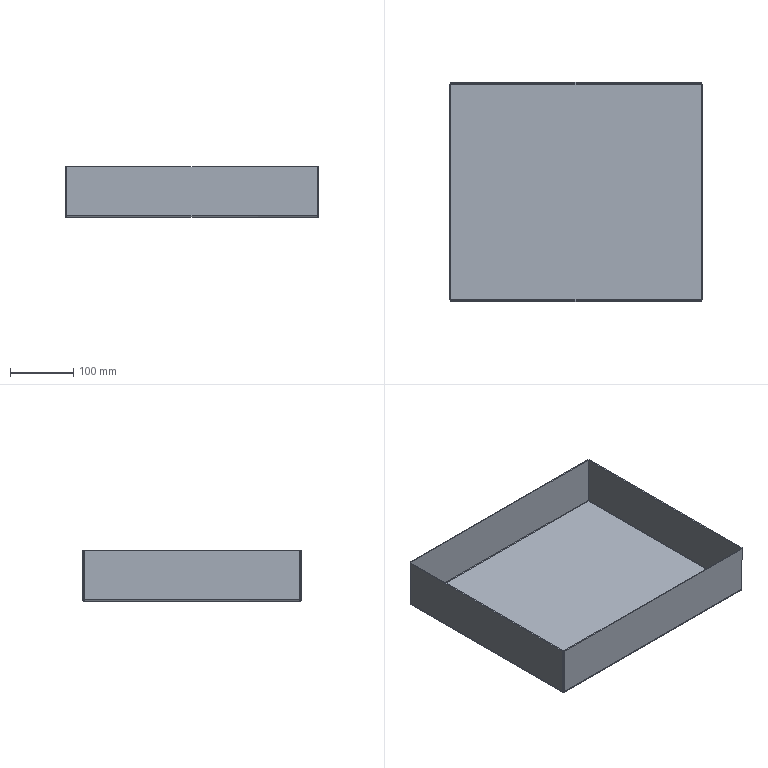Part | SolidWorks | features EdgeFlange 1, FlatPattern 1, SMBaseFlange 1, SheetMetal 1 | 1 solid | 38 faces | box 400 x 345 x 80 mm | volume 502813 mm3 | plane 22 | spline 8 | cylinder 8 | commonest cylinder face diameters 1.473 x4 5.473 x4
STEP:
#1=CARTESIAN_POINT('',(-197.263,169.763,-2.));
#2=VERTEX_POINT('',#1);
#3=CARTESIAN_POINT('',(197.263,169.763,-2.));
#4=VERTEX_POINT('',#3);
#5=CARTESIAN_POINT('',(-197.293,169.763,-2.));
#6=DIRECTION('',(1.,0.,0.));
#7=VECTOR('',#6,1000.);
#8=LINE('',#5,#7);
#9=EDGE_CURVE('',#2,#4,#8,.T.);
#10=ORIENTED_EDGE('',*,*,#9,.T.);
#11=CARTESIAN_POINT('',(197.263,-169.763,-2.));
#12=VERTEX_POINT('',#11);
#13=CARTESIAN_POINT('',(197.263,169.793,-2.));
#14=DIRECTION('',(0.,-1.,0.));
#15=VECTOR('',#14,1000.);
#16=LINE('',#13,#15);
#17=EDGE_CURVE('',#4,#12,#16,.T.);
#18=ORIENTED_EDGE('',*,*,#17,.T.);
#19=CARTESIAN_POINT('',(-197.263,-169.763,-2.));
#20=VERTEX_POINT('',#19);
#21=CARTESIAN_POINT('',(197.293,-169.763,-2.));
#22=DIRECTION('',(-1.,0.,0.));
#23=VECTOR('',#22,1000.);
#24=LINE('',#21,#23);
#25=EDGE_CURVE('',#12,#20,#24,.T.);
#26=ORIENTED_EDGE('',*,*,#25,.T.);
#27=CARTESIAN_POINT('',(-197.263,-169.793,-2.));
#28=DIRECTION('',(0.,1.,0.));
#29=VECTOR('',#28,1000.);
#30=LINE('',#27,#29);
#31=EDGE_CURVE('',#20,#2,#30,.T.);
#32=ORIENTED_EDGE('',*,*,#31,.T.);
#33=EDGE_LOOP('',(#10,#18,#26,#32));
#34=FACE_OUTER_BOUND('',#33,.T.);
#35=CARTESIAN_POINT('',(0.,0.,-2.));
#36=DIRECTION('',(0.,0.,-1.));
#37=DIRECTION('',(-1.,0.,0.));
#38=AXIS2_PLACEMENT_3D('',#35,#36,#37);
#39=PLANE('',#38);
#40=ADVANCED_FACE('',(#34),#39,.T.);
#41=CARTESIAN_POINT('',(197.263,169.763,0.));
#42=VERTEX_POINT('',#41);
#43=CARTESIAN_POINT('',(197.263,-169.763,0.));
#44=VERTEX_POINT('',#43);
#45=CARTESIAN_POINT('',(197.263,169.793,0.));
#46=DIRECTION('',(0.,-1.,0.));
#47=VECTOR('',#46,1000.);
#48=LINE('',#45,#47);
#49=EDGE_CURVE('',#42,#44,#48,.T.);
#50=ORIENTED_EDGE('',*,*,#49,.F.);
#51=CARTESIAN_POINT('',(-197.263,169.763,0.));
#52=VERTEX_POINT('',#51);
#53=CARTESIAN_POINT('',(-197.293,169.763,0.));
#54=DIRECTION('',(1.,0.,0.));
#55=VECTOR('',#54,1000.);
#56=LINE('',#53,#55);
#57=EDGE_CURVE('',#52,#42,#56,.T.);
#58=ORIENTED_EDGE('',*,*,#57,.F.);
#59=CARTESIAN_POINT('',(-197.263,-169.763,0.));
#60=VERTEX_POINT('',#59);
#61=CARTESIAN_POINT('',(-197.263,-169.793,0.));
#62=DIRECTION('',(0.,1.,0.));
#63=VECTOR('',#62,1000.);
#64=LINE('',#61,#63);
#65=EDGE_CURVE('',#60,#52,#64,.T.);
#66=ORIENTED_EDGE('',*,*,#65,.F.);
#67=CARTESIAN_POINT('',(197.293,-169.763,0.));
#68=DIRECTION('',(-1.,0.,0.));
#69=VECTOR('',#68,1000.);
#70=LINE('',#67,#69);
#71=EDGE_CURVE('',#44,#60,#70,.T.);
#72=ORIENTED_EDGE('',*,*,#71,.F.);
#73=EDGE_LOOP('',(#50,#58,#66,#72));
#74=FACE_OUTER_BOUND('',#73,.T.);
#75=CARTESIAN_POINT('',(0.,0.,0.));
#76=DIRECTION('',(0.,0.,-1.));
#77=DIRECTION('',(-1.,0.,0.));
#78=AXIS2_PLACEMENT_3D('',#75,#76,#77);
#79=PLANE('',#78);
#80=ADVANCED_FACE('',(#74),#79,.F.);
#81=CARTESIAN_POINT('',(197.293,172.5,0.7366));
#82=VERTEX_POINT('',#81);
#83=CARTESIAN_POINT('',(197.293,170.5,0.7366));
#84=VERTEX_POINT('',#83);
#85=CARTESIAN_POINT('',(197.293,170.5,0.7366));
#86=DIRECTION('',(0.,-1.,0.));
#87=VECTOR('',#86,1000.);
#88=LINE('',#85,#87);
#89=EDGE_CURVE('',#82,#84,#88,.T.);
#90=ORIENTED_EDGE('',*,*,#89,.T.);
#91=CARTESIAN_POINT('',(197.263,169.763,0.));
#92=CARTESIAN_POINT('',(197.268,169.956,0.));
#93=CARTESIAN_POINT('',(197.273,170.148,0.07939));
#94=CARTESIAN_POINT('',(197.283,170.421,0.3521));
#95=CARTESIAN_POINT('',(197.288,170.5,0.5438));
#96=CARTESIAN_POINT('',(197.293,170.5,0.7366));
#97=B_SPLINE_CURVE_WITH_KNOTS('',3,(#91,#92,#93,#94,#95,#96),.UNSPECIFIED.,.F.,.F.,(4,2,4),(0.,0.5,1.),.UNSPECIFIED.);
#98=EDGE_CURVE('',#42,#84,#97,.T.);
#99=ORIENTED_EDGE('',*,*,#98,.F.);
#100=CARTESIAN_POINT('',(197.263,169.763,0.));
#101=DIRECTION('',(0.,0.,-1.));
#102=VECTOR('',#101,1000.);
#103=LINE('',#100,#102);
#104=EDGE_CURVE('',#42,#4,#103,.T.);
#105=ORIENTED_EDGE('',*,*,#104,.T.);
#106=CARTESIAN_POINT('',(197.263,169.763,-2.));
#107=CARTESIAN_POINT('',(197.266,170.122,-2.));
#108=CARTESIAN_POINT('',(197.268,170.48,-1.929));
#109=CARTESIAN_POINT('',(197.273,171.142,-1.655));
#110=CARTESIAN_POINT('',(197.276,171.445,-1.452));
#111=CARTESIAN_POINT('',(197.281,171.952,-0.9452));
#112=CARTESIAN_POINT('',(197.283,172.155,-0.6416));
#113=CARTESIAN_POINT('',(197.288,172.429,0.0203));
#114=CARTESIAN_POINT('',(197.29,172.5,0.3784));
#115=CARTESIAN_POINT('',(197.293,172.5,0.7366));
#116=B_SPLINE_CURVE_WITH_KNOTS('',3,(#106,#107,#108,#109,#110,#111,#112,#113,#114,#115),.UNSPECIFIED.,.F.,.F.,(4,2,2,2,4),(0.,0.25,0.5,0.75,1.),.UNSPECIFIED.);
#117=EDGE_CURVE('',#4,#82,#116,.T.);
#118=ORIENTED_EDGE('',*,*,#117,.T.);
#119=EDGE_LOOP('',(#90,#99,#105,#118));
#120=FACE_OUTER_BOUND('',#119,.T.);
#121=CARTESIAN_POINT('',(197.263,169.763,-2.02));
#122=CARTESIAN_POINT('',(197.266,170.124,-2.02));
#123=CARTESIAN_POINT('',(197.268,170.485,-1.948));
#124=CARTESIAN_POINT('',(197.273,171.152,-1.672));
#125=CARTESIAN_POINT('',(197.276,171.457,-1.468));
#126=CARTESIAN_POINT('',(197.281,171.968,-0.9575));
#127=CARTESIAN_POINT('',(197.283,172.172,-0.6517));
#128=CARTESIAN_POINT('',(197.288,172.448,0.01507));
#129=CARTESIAN_POINT('',(197.29,172.52,0.3757));
#130=CARTESIAN_POINT('',(197.293,172.52,0.7366));
#131=CARTESIAN_POINT('',(197.263,169.763,-2.));
#132=CARTESIAN_POINT('',(197.266,170.122,-2.));
#133=CARTESIAN_POINT('',(197.268,170.48,-1.929));
#134=CARTESIAN_POINT('',(197.273,171.142,-1.655));
#135=CARTESIAN_POINT('',(197.276,171.445,-1.452));
#136=CARTESIAN_POINT('',(197.281,171.952,-0.9452));
#137=CARTESIAN_POINT('',(197.283,172.155,-0.6416));
#138=CARTESIAN_POINT('',(197.288,172.429,0.0203));
#139=CARTESIAN_POINT('',(197.29,172.5,0.3783));
#140=CARTESIAN_POINT('',(197.293,172.5,0.7366));
#141=CARTESIAN_POINT('',(197.263,169.763,0.));
#142=CARTESIAN_POINT('',(197.266,169.86,0.));
#143=CARTESIAN_POINT('',(197.268,169.956,0.01917));
#144=CARTESIAN_POINT('',(197.273,170.134,0.09297));
#145=CARTESIAN_POINT('',(197.276,170.216,0.1476));
#146=CARTESIAN_POINT('',(197.281,170.352,0.2839));
#147=CARTESIAN_POINT('',(197.283,170.407,0.3656));
#148=CARTESIAN_POINT('',(197.288,170.481,0.5438));
#149=CARTESIAN_POINT('',(197.29,170.5,0.6402));
#150=CARTESIAN_POINT('',(197.293,170.5,0.7366));
#151=CARTESIAN_POINT('',(197.263,169.763,0.0202));
#152=CARTESIAN_POINT('',(197.266,169.857,0.0202));
#153=CARTESIAN_POINT('',(197.268,169.951,0.03885));
#154=CARTESIAN_POINT('',(197.273,170.124,0.1106));
#155=CARTESIAN_POINT('',(197.276,170.204,0.1637));
#156=CARTESIAN_POINT('',(197.281,170.336,0.2963));
#157=CARTESIAN_POINT('',(197.283,170.389,0.3758));
#158=CARTESIAN_POINT('',(197.288,170.461,0.5491));
#159=CARTESIAN_POINT('',(197.29,170.48,0.6428));
#160=CARTESIAN_POINT('',(197.293,170.48,0.7366));
#161=B_SPLINE_SURFACE_WITH_KNOTS('',1,3,((#121,#122,#123,#124,#125,#126,#127,#128,#129,#130),(#131,#132,#133,#134,#135,#136,#137,#138,#139,#140),(#141,#142,#143,#144,#145,#146,#147,#148,#149,#150),(#151,#152,#153,#154,#155,#156,#157,#158,#159,#160)),.UNSPECIFIED.,.F.,.F.,.F.,(2,1,1,2),(4,2,2,2,4),(-0.01,0.,1.,1.01),(0.,0.25,0.5,0.75,1.),.UNSPECIFIED.);
#162=ADVANCED_FACE('',(#120),#161,.F.);
#163=CARTESIAN_POINT('',(-197.293,170.5,0.7366));
#164=VERTEX_POINT('',#163);
#165=CARTESIAN_POINT('',(-197.293,170.5,0.7366));
#166=CARTESIAN_POINT('',(-197.288,170.5,0.5438));
#167=CARTESIAN_POINT('',(-197.283,170.421,0.3521));
#168=CARTESIAN_POINT('',(-197.273,170.148,0.07939));
#169=CARTESIAN_POINT('',(-197.268,169.956,0.));
#170=CARTESIAN_POINT('',(-197.263,169.763,0.));
#171=B_SPLINE_CURVE_WITH_KNOTS('',3,(#165,#166,#167,#168,#169,#170),.UNSPECIFIED.,.F.,.F.,(4,2,4),(0.,0.5,1.),.UNSPECIFIED.);
#172=EDGE_CURVE('',#164,#52,#171,.T.);
#173=ORIENTED_EDGE('',*,*,#172,.F.);
#174=CARTESIAN_POINT('',(-197.293,172.5,0.7366));
#175=VERTEX_POINT('',#174);
#176=CARTESIAN_POINT('',(-197.293,170.5,0.7366));
#177=DIRECTION('',(0.,-1.,0.));
#178=VECTOR('',#177,1000.);
#179=LINE('',#176,#178);
#180=EDGE_CURVE('',#175,#164,#179,.T.);
#181=ORIENTED_EDGE('',*,*,#180,.F.);
#182=CARTESIAN_POINT('',(-197.293,172.5,0.7366));
#183=CARTESIAN_POINT('',(-197.29,172.5,0.3784));
#184=CARTESIAN_POINT('',(-197.288,172.429,0.0203));
#185=CARTESIAN_POINT('',(-197.283,172.155,-0.6416));
#186=CARTESIAN_POINT('',(-197.281,171.952,-0.9452));
#187=CARTESIAN_POINT('',(-197.276,171.445,-1.452));
#188=CARTESIAN_POINT('',(-197.273,171.142,-1.655));
#189=CARTESIAN_POINT('',(-197.268,170.48,-1.929));
#190=CARTESIAN_POINT('',(-197.266,170.122,-2.));
#191=CARTESIAN_POINT('',(-197.263,169.763,-2.));
#192=B_SPLINE_CURVE_WITH_KNOTS('',3,(#182,#183,#184,#185,#186,#187,#188,#189,#190,#191),.UNSPECIFIED.,.F.,.F.,(4,2,2,2,4),(0.,0.25,0.5,0.75,1.),.UNSPECIFIED.);
#193=EDGE_CURVE('',#175,#2,#192,.T.);
#194=ORIENTED_EDGE('',*,*,#193,.T.);
#195=CARTESIAN_POINT('',(-197.263,169.763,0.));
#196=DIRECTION('',(0.,0.,-1.));
#197=VECTOR('',#196,1000.);
#198=LINE('',#195,#197);
#199=EDGE_CURVE('',#52,#2,#198,.T.);
#200=ORIENTED_EDGE('',*,*,#199,.F.);
#201=EDGE_LOOP('',(#173,#181,#194,#200));
#202=FACE_OUTER_BOUND('',#201,.T.);
#203=CARTESIAN_POINT('',(-197.293,172.52,0.7366));
#204=CARTESIAN_POINT('',(-197.29,172.52,0.3757));
#205=CARTESIAN_POINT('',(-197.288,172.448,0.01507));
#206=CARTESIAN_POINT('',(-197.283,172.172,-0.6517));
#207=CARTESIAN_POINT('',(-197.281,171.968,-0.9575));
#208=CARTESIAN_POINT('',(-197.276,171.457,-1.468));
#209=CARTESIAN_POINT('',(-197.273,171.152,-1.672));
#210=CARTESIAN_POINT('',(-197.268,170.485,-1.948));
#211=CARTESIAN_POINT('',(-197.266,170.124,-2.02));
#212=CARTESIAN_POINT('',(-197.263,169.763,-2.02));
#213=CARTESIAN_POINT('',(-197.293,172.5,0.7366));
#214=CARTESIAN_POINT('',(-197.29,172.5,0.3783));
#215=CARTESIAN_POINT('',(-197.288,172.429,0.0203));
#216=CARTESIAN_POINT('',(-197.283,172.155,-0.6416));
#217=CARTESIAN_POINT('',(-197.281,171.952,-0.9452));
#218=CARTESIAN_POINT('',(-197.276,171.445,-1.452));
#219=CARTESIAN_POINT('',(-197.273,171.142,-1.655));
#220=CARTESIAN_POINT('',(-197.268,170.48,-1.929));
#221=CARTESIAN_POINT('',(-197.266,170.122,-2.));
#222=CARTESIAN_POINT('',(-197.263,169.763,-2.));
#223=CARTESIAN_POINT('',(-197.293,170.5,0.7366));
#224=CARTESIAN_POINT('',(-197.29,170.5,0.6402));
#225=CARTESIAN_POINT('',(-197.288,170.481,0.5438));
#226=CARTESIAN_POINT('',(-197.283,170.407,0.3656));
#227=CARTESIAN_POINT('',(-197.281,170.352,0.2839));
#228=CARTESIAN_POINT('',(-197.276,170.216,0.1476));
#229=CARTESIAN_POINT('',(-197.273,170.134,0.09297));
#230=CARTESIAN_POINT('',(-197.268,169.956,0.01917));
#231=CARTESIAN_POINT('',(-197.266,169.86,0.));
#232=CARTESIAN_POINT('',(-197.263,169.763,0.));
#233=CARTESIAN_POINT('',(-197.293,170.48,0.7366));
#234=CARTESIAN_POINT('',(-197.29,170.48,0.6428));
#235=CARTESIAN_POINT('',(-197.288,170.461,0.5491));
#236=CARTESIAN_POINT('',(-197.283,170.389,0.3758));
#237=CARTESIAN_POINT('',(-197.281,170.336,0.2963));
#238=CARTESIAN_POINT('',(-197.276,170.204,0.1637));
#239=CARTESIAN_POINT('',(-197.273,170.124,0.1106));
#240=CARTESIAN_POINT('',(-197.268,169.951,0.03885));
#241=CARTESIAN_POINT('',(-197.266,169.857,0.0202));
#242=CARTESIAN_POINT('',(-197.263,169.763,0.0202));
#243=B_SPLINE_SURFACE_WITH_KNOTS('',1,3,((#203,#204,#205,#206,#207,#208,#209,#210,#211,#212),(#213,#214,#215,#216,#217,#218,#219,#220,#221,#222),(#223,#224,#225,#226,#227,#228,#229,#230,#231,#232),(#233,#234,#235,#236,#237,#238,#239,#240,#241,#242)),.UNSPECIFIED.,.F.,.F.,.F.,(2,1,1,2),(4,2,2,2,4),(-0.01,0.,1.,1.01),(0.,0.25,0.5,0.75,1.),.UNSPECIFIED.);
#244=ADVANCED_FACE('',(#202),#243,.F.);
#245=ORIENTED_EDGE('',*,*,#9,.F.);
#246=ORIENTED_EDGE('',*,*,#193,.F.);
#247=CARTESIAN_POINT('',(200.,172.5,0.7366));
#248=DIRECTION('',(1.,0.,0.));
#249=VECTOR('',#248,1000.);
#250=LINE('',#247,#249);
#251=EDGE_CURVE('',#175,#82,#250,.T.);
#252=ORIENTED_EDGE('',*,*,#251,.T.);
#253=ORIENTED_EDGE('',*,*,#117,.F.);
#254=EDGE_LOOP('',(#245,#246,#252,#253));
#255=FACE_OUTER_BOUND('',#254,.T.);
#256=CARTESIAN_POINT('',(-197.293,169.763,0.7366));
#257=DIRECTION('',(-1.,0.,0.));
#258=DIRECTION('',(0.,1.,0.));
#259=AXIS2_PLACEMENT_3D('',#256,#257,#258);
#260=CYLINDRICAL_SURFACE('',#259,2.737);
#261=ADVANCED_FACE('',(#255),#260,.T.);
#262=ORIENTED_EDGE('',*,*,#57,.T.);
#263=ORIENTED_EDGE('',*,*,#98,.T.);
#264=CARTESIAN_POINT('',(200.,170.5,0.7366));
#265=DIRECTION('',(-1.,0.,0.));
#266=VECTOR('',#265,1000.);
#267=LINE('',#264,#266);
#268=EDGE_CURVE('',#84,#164,#267,.T.);
#269=ORIENTED_EDGE('',*,*,#268,.T.);
#270=ORIENTED_EDGE('',*,*,#172,.T.);
#271=EDGE_LOOP('',(#262,#263,#269,#270));
#272=FACE_OUTER_BOUND('',#271,.T.);
#273=CARTESIAN_POINT('',(-197.293,169.763,0.7366));
#274=DIRECTION('',(-1.,0.,0.));
#275=DIRECTION('',(0.,1.,0.));
#276=AXIS2_PLACEMENT_3D('',#273,#274,#275);
#277=CYLINDRICAL_SURFACE('',#276,0.7366);
#278=ADVANCED_FACE('',(#272),#277,.F.);
#279=CARTESIAN_POINT('',(197.293,172.5,78.));
#280=VERTEX_POINT('',#279);
#281=CARTESIAN_POINT('',(197.293,172.5,0.));
#282=DIRECTION('',(0.,0.,1.));
#283=VECTOR('',#282,1000.);
#284=LINE('',#281,#283);
#285=EDGE_CURVE('',#82,#280,#284,.T.);
#286=ORIENTED_EDGE('',*,*,#285,.T.);
#287=CARTESIAN_POINT('',(197.293,170.5,78.));
#288=VERTEX_POINT('',#287);
#289=CARTESIAN_POINT('',(197.293,170.5,78.));
#290=DIRECTION('',(0.,-1.,0.));
#291=VECTOR('',#290,1000.);
#292=LINE('',#289,#291);
#293=EDGE_CURVE('',#280,#288,#292,.T.);
#294=ORIENTED_EDGE('',*,*,#293,.T.);
#295=CARTESIAN_POINT('',(197.293,170.5,0.));
#296=DIRECTION('',(0.,0.,1.));
#297=VECTOR('',#296,1000.);
#298=LINE('',#295,#297);
#299=EDGE_CURVE('',#84,#288,#298,.T.);
#300=ORIENTED_EDGE('',*,*,#299,.F.);
#301=ORIENTED_EDGE('',*,*,#89,.F.);
#302=EDGE_LOOP('',(#286,#294,#300,#301));
#303=FACE_OUTER_BOUND('',#302,.T.);
#304=CARTESIAN_POINT('',(197.293,170.5,0.));
#305=DIRECTION('',(1.,0.,0.));
#306=DIRECTION('',(0.,0.,-1.));
#307=AXIS2_PLACEMENT_3D('',#304,#305,#306);
#308=PLANE('',#307);
#309=ADVANCED_FACE('',(#303),#308,.T.);
#310=ORIENTED_EDGE('',*,*,#251,.F.);
#311=CARTESIAN_POINT('',(-197.293,172.5,78.));
#312=VERTEX_POINT('',#311);
#313=CARTESIAN_POINT('',(-197.293,172.5,0.));
#314=DIRECTION('',(0.,0.,1.));
#315=VECTOR('',#314,1000.);
#316=LINE('',#313,#315);
#317=EDGE_CURVE('',#175,#312,#316,.T.);
#318=ORIENTED_EDGE('',*,*,#317,.T.);
#319=CARTESIAN_POINT('',(0.,172.5,78.));
#320=DIRECTION('',(1.,0.,0.));
#321=VECTOR('',#320,1000.);
#322=LINE('',#319,#321);
#323=EDGE_CURVE('',#312,#280,#322,.T.);
#324=ORIENTED_EDGE('',*,*,#323,.T.);
#325=ORIENTED_EDGE('',*,*,#285,.F.);
#326=EDGE_LOOP('',(#310,#318,#324,#325));
#327=FACE_OUTER_BOUND('',#326,.T.);
#328=CARTESIAN_POINT('',(0.,172.5,0.));
#329=DIRECTION('',(0.,-1.,0.));
#330=DIRECTION('',(0.,0.,-1.));
#331=AXIS2_PLACEMENT_3D('',#328,#329,#330);
#332=PLANE('',#331);
#333=ADVANCED_FACE('',(#327),#332,.F.);
#334=CARTESIAN_POINT('',(-197.293,170.5,78.));
#335=VERTEX_POINT('',#334);
#336=CARTESIAN_POINT('',(-197.293,170.5,0.));
#337=DIRECTION('',(0.,0.,1.));
#338=VECTOR('',#337,1000.);
#339=LINE('',#336,#338);
#340=EDGE_CURVE('',#164,#335,#339,.T.);
#341=ORIENTED_EDGE('',*,*,#340,.F.);
#342=ORIENTED_EDGE('',*,*,#268,.F.);
#343=ORIENTED_EDGE('',*,*,#299,.T.);
#344=CARTESIAN_POINT('',(200.,170.5,78.));
#345=DIRECTION('',(1.,0.,0.));
#346=VECTOR('',#345,1000.);
#347=LINE('',#344,#346);
#348=EDGE_CURVE('',#335,#288,#347,.T.);
#349=ORIENTED_EDGE('',*,*,#348,.F.);
#350=EDGE_LOOP('',(#341,#342,#343,#349));
#351=FACE_OUTER_BOUND('',#350,.T.);
#352=CARTESIAN_POINT('',(0.,170.5,0.));
#353=DIRECTION('',(0.,-1.,0.));
#354=DIRECTION('',(0.,0.,-1.));
#355=AXIS2_PLACEMENT_3D('',#352,#353,#354);
#356=PLANE('',#355);
#357=ADVANCED_FACE('',(#351),#356,.T.);
#358=ORIENTED_EDGE('',*,*,#323,.F.);
#359=CARTESIAN_POINT('',(-197.293,172.5,78.));
#360=DIRECTION('',(0.,-1.,0.));
#361=VECTOR('',#360,1000.);
#362=LINE('',#359,#361);
#363=EDGE_CURVE('',#312,#335,#362,.T.);
#364=ORIENTED_EDGE('',*,*,#363,.T.);
#365=ORIENTED_EDGE('',*,*,#348,.T.);
#366=ORIENTED_EDGE('',*,*,#293,.F.);
#367=EDGE_LOOP('',(#358,#364,#365,#366));
#368=FACE_OUTER_BOUND('',#367,.T.);
#369=CARTESIAN_POINT('',(200.,172.5,78.));
#370=DIRECTION('',(0.,0.,-1.));
#371=DIRECTION('',(0.,1.,0.));
#372=AXIS2_PLACEMENT_3D('',#369,#370,#371);
#373=PLANE('',#372);
#374=ADVANCED_FACE('',(#368),#373,.F.);
#375=ORIENTED_EDGE('',*,*,#363,.F.);
#376=ORIENTED_EDGE('',*,*,#317,.F.);
#377=ORIENTED_EDGE('',*,*,#180,.T.);
#378=ORIENTED_EDGE('',*,*,#340,.T.);
#379=EDGE_LOOP('',(#375,#376,#377,#378));
#380=FACE_OUTER_BOUND('',#379,.T.);
#381=CARTESIAN_POINT('',(-197.293,170.5,0.));
#382=DIRECTION('',(1.,0.,0.));
#383=DIRECTION('',(0.,0.,-1.));
#384=AXIS2_PLACEMENT_3D('',#381,#382,#383);
#385=PLANE('',#384);
#386=ADVANCED_FACE('',(#380),#385,.F.);
#387=CARTESIAN_POINT('',(-200.,169.793,0.7366));
#388=VERTEX_POINT('',#387);
#389=CARTESIAN_POINT('',(-198.,169.793,0.7366));
#390=VERTEX_POINT('',#389);
#391=CARTESIAN_POINT('',(-198.,169.793,0.7366));
#392=DIRECTION('',(1.,0.,0.));
#393=VECTOR('',#392,1000.);
#394=LINE('',#391,#393);
#395=EDGE_CURVE('',#388,#390,#394,.T.);
#396=ORIENTED_EDGE('',*,*,#395,.T.);
#397=CARTESIAN_POINT('',(-197.263,169.763,0.));
#398=CARTESIAN_POINT('',(-197.456,169.768,0.));
#399=CARTESIAN_POINT('',(-197.648,169.773,0.07939));
#400=CARTESIAN_POINT('',(-197.921,169.783,0.3521));
#401=CARTESIAN_POINT('',(-198.,169.788,0.5438));
#402=CARTESIAN_POINT('',(-198.,169.793,0.7366));
#403=B_SPLINE_CURVE_WITH_KNOTS('',3,(#397,#398,#399,#400,#401,#402),.UNSPECIFIED.,.F.,.F.,(4,2,4),(0.,0.5,1.),.UNSPECIFIED.);
#404=EDGE_CURVE('',#52,#390,#403,.T.);
#405=ORIENTED_EDGE('',*,*,#404,.F.);
#406=ORIENTED_EDGE('',*,*,#199,.T.);
#407=CARTESIAN_POINT('',(-197.263,169.763,-2.));
#408=CARTESIAN_POINT('',(-197.622,169.766,-2.));
#409=CARTESIAN_POINT('',(-197.98,169.768,-1.929));
#410=CARTESIAN_POINT('',(-198.642,169.773,-1.655));
#411=CARTESIAN_POINT('',(-198.945,169.776,-1.452));
#412=CARTESIAN_POINT('',(-199.452,169.781,-0.9452));
#413=CARTESIAN_POINT('',(-199.655,169.783,-0.6416));
#414=CARTESIAN_POINT('',(-199.929,169.788,0.0203));
#415=CARTESIAN_POINT('',(-200.,169.79,0.3784));
#416=CARTESIAN_POINT('',(-200.,169.793,0.7366));
#417=B_SPLINE_CURVE_WITH_KNOTS('',3,(#407,#408,#409,#410,#411,#412,#413,#414,#415,#416),.UNSPECIFIED.,.F.,.F.,(4,2,2,2,4),(0.,0.25,0.5,0.75,1.),.UNSPECIFIED.);
#418=EDGE_CURVE('',#2,#388,#417,.T.);
#419=ORIENTED_EDGE('',*,*,#418,.T.);
#420=EDGE_LOOP('',(#396,#405,#406,#419));
#421=FACE_OUTER_BOUND('',#420,.T.);
#422=CARTESIAN_POINT('',(-197.263,169.763,-2.02));
#423=CARTESIAN_POINT('',(-197.624,169.766,-2.02));
#424=CARTESIAN_POINT('',(-197.985,169.768,-1.948));
#425=CARTESIAN_POINT('',(-198.652,169.773,-1.672));
#426=CARTESIAN_POINT('',(-198.957,169.776,-1.468));
#427=CARTESIAN_POINT('',(-199.468,169.781,-0.9575));
#428=CARTESIAN_POINT('',(-199.672,169.783,-0.6517));
#429=CARTESIAN_POINT('',(-199.948,169.788,0.01507));
#430=CARTESIAN_POINT('',(-200.02,169.79,0.3757));
#431=CARTESIAN_POINT('',(-200.02,169.793,0.7366));
#432=CARTESIAN_POINT('',(-197.263,169.763,-2.));
#433=CARTESIAN_POINT('',(-197.622,169.766,-2.));
#434=CARTESIAN_POINT('',(-197.98,169.768,-1.929));
#435=CARTESIAN_POINT('',(-198.642,169.773,-1.655));
#436=CARTESIAN_POINT('',(-198.945,169.776,-1.452));
#437=CARTESIAN_POINT('',(-199.452,169.781,-0.9452));
#438=CARTESIAN_POINT('',(-199.655,169.783,-0.6416));
#439=CARTESIAN_POINT('',(-199.929,169.788,0.0203));
#440=CARTESIAN_POINT('',(-200.,169.79,0.3783));
#441=CARTESIAN_POINT('',(-200.,169.793,0.7366));
#442=CARTESIAN_POINT('',(-197.263,169.763,0.));
#443=CARTESIAN_POINT('',(-197.36,169.766,0.));
#444=CARTESIAN_POINT('',(-197.456,169.768,0.01917));
#445=CARTESIAN_POINT('',(-197.634,169.773,0.09297));
#446=CARTESIAN_POINT('',(-197.716,169.776,0.1476));
#447=CARTESIAN_POINT('',(-197.852,169.781,0.2839));
#448=CARTESIAN_POINT('',(-197.907,169.783,0.3656));
#449=CARTESIAN_POINT('',(-197.981,169.788,0.5438));
#450=CARTESIAN_POINT('',(-198.,169.79,0.6402));
#451=CARTESIAN_POINT('',(-198.,169.793,0.7366));
#452=CARTESIAN_POINT('',(-197.263,169.763,0.0202));
#453=CARTESIAN_POINT('',(-197.357,169.766,0.0202));
#454=CARTESIAN_POINT('',(-197.451,169.768,0.03885));
#455=CARTESIAN_POINT('',(-197.624,169.773,0.1106));
#456=CARTESIAN_POINT('',(-197.704,169.776,0.1637));
#457=CARTESIAN_POINT('',(-197.836,169.781,0.2963));
#458=CARTESIAN_POINT('',(-197.889,169.783,0.3758));
#459=CARTESIAN_POINT('',(-197.961,169.788,0.5491));
#460=CARTESIAN_POINT('',(-197.98,169.79,0.6428));
#461=CARTESIAN_POINT('',(-197.98,169.793,0.7366));
#462=B_SPLINE_SURFACE_WITH_KNOTS('',1,3,((#422,#423,#424,#425,#426,#427,#428,#429,#430,#431),(#432,#433,#434,#435,#436,#437,#438,#439,#440,#441),(#442,#443,#444,#445,#446,#447,#448,#449,#450,#451),(#452,#453,#454,#455,#456,#457,#458,#459,#460,#461)),.UNSPECIFIED.,.F.,.F.,.F.,(2,1,1,2),(4,2,2,2,4),(-0.01,0.,1.,1.01),(0.,0.25,0.5,0.75,1.),.UNSPECIFIED.);
#463=ADVANCED_FACE('',(#421),#462,.F.);
#464=CARTESIAN_POINT('',(-198.,-169.793,0.7366));
#465=VERTEX_POINT('',#464);
#466=CARTESIAN_POINT('',(-198.,-169.793,0.7366));
#467=CARTESIAN_POINT('',(-198.,-169.788,0.5438));
#468=CARTESIAN_POINT('',(-197.921,-169.783,0.3521));
#469=CARTESIAN_POINT('',(-197.648,-169.773,0.07939));
#470=CARTESIAN_POINT('',(-197.456,-169.768,0.));
#471=CARTESIAN_POINT('',(-197.263,-169.763,0.));
#472=B_SPLINE_CURVE_WITH_KNOTS('',3,(#466,#467,#468,#469,#470,#471),.UNSPECIFIED.,.F.,.F.,(4,2,4),(0.,0.5,1.),.UNSPECIFIED.);
#473=EDGE_CURVE('',#465,#60,#472,.T.);
#474=ORIENTED_EDGE('',*,*,#473,.F.);
#475=CARTESIAN_POINT('',(-200.,-169.793,0.7366));
#476=VERTEX_POINT('',#475);
#477=CARTESIAN_POINT('',(-198.,-169.793,0.7366));
#478=DIRECTION('',(1.,0.,0.));
#479=VECTOR('',#478,1000.);
#480=LINE('',#477,#479);
#481=EDGE_CURVE('',#476,#465,#480,.T.);
#482=ORIENTED_EDGE('',*,*,#481,.F.);
#483=CARTESIAN_POINT('',(-200.,-169.793,0.7366));
#484=CARTESIAN_POINT('',(-200.,-169.79,0.3784));
#485=CARTESIAN_POINT('',(-199.929,-169.788,0.0203));
#486=CARTESIAN_POINT('',(-199.655,-169.783,-0.6416));
#487=CARTESIAN_POINT('',(-199.452,-169.781,-0.9452));
#488=CARTESIAN_POINT('',(-198.945,-169.776,-1.452));
#489=CARTESIAN_POINT('',(-198.642,-169.773,-1.655));
#490=CARTESIAN_POINT('',(-197.98,-169.768,-1.929));
#491=CARTESIAN_POINT('',(-197.622,-169.766,-2.));
#492=CARTESIAN_POINT('',(-197.263,-169.763,-2.));
#493=B_SPLINE_CURVE_WITH_KNOTS('',3,(#483,#484,#485,#486,#487,#488,#489,#490,#491,#492),.UNSPECIFIED.,.F.,.F.,(4,2,2,2,4),(0.,0.25,0.5,0.75,1.),.UNSPECIFIED.);
#494=EDGE_CURVE('',#476,#20,#493,.T.);
#495=ORIENTED_EDGE('',*,*,#494,.T.);
#496=CARTESIAN_POINT('',(-197.263,-169.763,0.));
#497=DIRECTION('',(0.,0.,-1.));
#498=VECTOR('',#497,1000.);
#499=LINE('',#496,#498);
#500=EDGE_CURVE('',#60,#20,#499,.T.);
#501=ORIENTED_EDGE('',*,*,#500,.F.);
#502=EDGE_LOOP('',(#474,#482,#495,#501));
#503=FACE_OUTER_BOUND('',#502,.T.);
#504=CARTESIAN_POINT('',(-200.02,-169.793,0.7366));
#505=CARTESIAN_POINT('',(-200.02,-169.79,0.3757));
#506=CARTESIAN_POINT('',(-199.948,-169.788,0.01507));
#507=CARTESIAN_POINT('',(-199.672,-169.783,-0.6517));
#508=CARTESIAN_POINT('',(-199.468,-169.781,-0.9575));
#509=CARTESIAN_POINT('',(-198.957,-169.776,-1.468));
#510=CARTESIAN_POINT('',(-198.652,-169.773,-1.672));
#511=CARTESIAN_POINT('',(-197.985,-169.768,-1.948));
#512=CARTESIAN_POINT('',(-197.624,-169.766,-2.02));
#513=CARTESIAN_POINT('',(-197.263,-169.763,-2.02));
#514=CARTESIAN_POINT('',(-200.,-169.793,0.7366));
#515=CARTESIAN_POINT('',(-200.,-169.79,0.3783));
#516=CARTESIAN_POINT('',(-199.929,-169.788,0.0203));
#517=CARTESIAN_POINT('',(-199.655,-169.783,-0.6416));
#518=CARTESIAN_POINT('',(-199.452,-169.781,-0.9452));
#519=CARTESIAN_POINT('',(-198.945,-169.776,-1.452));
#520=CARTESIAN_POINT('',(-198.642,-169.773,-1.655));
#521=CARTESIAN_POINT('',(-197.98,-169.768,-1.929));
#522=CARTESIAN_POINT('',(-197.622,-169.766,-2.));
#523=CARTESIAN_POINT('',(-197.263,-169.763,-2.));
#524=CARTESIAN_POINT('',(-198.,-169.793,0.7366));
#525=CARTESIAN_POINT('',(-198.,-169.79,0.6402));
#526=CARTESIAN_POINT('',(-197.981,-169.788,0.5438));
#527=CARTESIAN_POINT('',(-197.907,-169.783,0.3656));
#528=CARTESIAN_POINT('',(-197.852,-169.781,0.2839));
#529=CARTESIAN_POINT('',(-197.716,-169.776,0.1476));
#530=CARTESIAN_POINT('',(-197.634,-169.773,0.09297));
#531=CARTESIAN_POINT('',(-197.456,-169.768,0.01917));
#532=CARTESIAN_POINT('',(-197.36,-169.766,0.));
#533=CARTESIAN_POINT('',(-197.263,-169.763,0.));
#534=CARTESIAN_POINT('',(-197.98,-169.793,0.7366));
#535=CARTESIAN_POINT('',(-197.98,-169.79,0.6428));
#536=CARTESIAN_POINT('',(-197.961,-169.788,0.5491));
#537=CARTESIAN_POINT('',(-197.889,-169.783,0.3758));
#538=CARTESIAN_POINT('',(-197.836,-169.781,0.2963));
#539=CARTESIAN_POINT('',(-197.704,-169.776,0.1637));
#540=CARTESIAN_POINT('',(-197.624,-169.773,0.1106));
#541=CARTESIAN_POINT('',(-197.451,-169.768,0.03885));
#542=CARTESIAN_POINT('',(-197.357,-169.766,0.0202));
#543=CARTESIAN_POINT('',(-197.263,-169.763,0.0202));
#544=B_SPLINE_SURFACE_WITH_KNOTS('',1,3,((#504,#505,#506,#507,#508,#509,#510,#511,#512,#513),(#514,#515,#516,#517,#518,#519,#520,#521,#522,#523),(#524,#525,#526,#527,#528,#529,#530,#531,#532,#533),(#534,#535,#536,#537,#538,#539,#540,#541,#542,#543)),.UNSPECIFIED.,.F.,.F.,.F.,(2,1,1,2),(4,2,2,2,4),(-0.01,0.,1.,1.01),(0.,0.25,0.5,0.75,1.),.UNSPECIFIED.);
#545=ADVANCED_FACE('',(#503),#544,.F.);
#546=ORIENTED_EDGE('',*,*,#31,.F.);
#547=ORIENTED_EDGE('',*,*,#494,.F.);
#548=CARTESIAN_POINT('',(-200.,172.5,0.7366));
#549=DIRECTION('',(0.,1.,0.));
#550=VECTOR('',#549,1000.);
#551=LINE('',#548,#550);
#552=EDGE_CURVE('',#476,#388,#551,.T.);
#553=ORIENTED_EDGE('',*,*,#552,.T.);
#554=ORIENTED_EDGE('',*,*,#418,.F.);
#555=EDGE_LOOP('',(#546,#547,#553,#554));
#556=FACE_OUTER_BOUND('',#555,.T.);
#557=CARTESIAN_POINT('',(-197.263,-169.793,0.7366));
#558=DIRECTION('',(0.,-1.,0.));
#559=DIRECTION('',(-1.,0.,0.));
#560=AXIS2_PLACEMENT_3D('',#557,#558,#559);
#561=CYLINDRICAL_SURFACE('',#560,2.737);
#562=ADVANCED_FACE('',(#556),#561,.T.);
#563=ORIENTED_EDGE('',*,*,#65,.T.);
#564=ORIENTED_EDGE('',*,*,#404,.T.);
#565=CARTESIAN_POINT('',(-198.,172.5,0.7366));
#566=DIRECTION('',(0.,-1.,0.));
#567=VECTOR('',#566,1000.);
#568=LINE('',#565,#567);
#569=EDGE_CURVE('',#390,#465,#568,.T.);
#570=ORIENTED_EDGE('',*,*,#569,.T.);
#571=ORIENTED_EDGE('',*,*,#473,.T.);
#572=EDGE_LOOP('',(#563,#564,#570,#571));
#573=FACE_OUTER_BOUND('',#572,.T.);
#574=CARTESIAN_POINT('',(-197.263,-169.793,0.7366));
#575=DIRECTION('',(0.,-1.,0.));
#576=DIRECTION('',(-1.,0.,0.));
#577=AXIS2_PLACEMENT_3D('',#574,#575,#576);
#578=CYLINDRICAL_SURFACE('',#577,0.7366);
#579=ADVANCED_FACE('',(#573),#578,.F.);
#580=CARTESIAN_POINT('',(-200.,169.793,78.));
#581=VERTEX_POINT('',#580);
#582=CARTESIAN_POINT('',(-200.,169.793,0.));
#583=DIRECTION('',(0.,0.,1.));
#584=VECTOR('',#583,1000.);
#585=LINE('',#582,#584);
#586=EDGE_CURVE('',#388,#581,#585,.T.);
#587=ORIENTED_EDGE('',*,*,#586,.T.);
#588=CARTESIAN_POINT('',(-198.,169.793,78.));
#589=VERTEX_POINT('',#588);
#590=CARTESIAN_POINT('',(-198.,169.793,78.));
#591=DIRECTION('',(1.,0.,0.));
#592=VECTOR('',#591,1000.);
#593=LINE('',#590,#592);
#594=EDGE_CURVE('',#581,#589,#593,.T.);
#595=ORIENTED_EDGE('',*,*,#594,.T.);
#596=CARTESIAN_POINT('',(-198.,169.793,0.));
#597=DIRECTION('',(0.,0.,1.));
#598=VECTOR('',#597,1000.);
#599=LINE('',#596,#598);
#600=EDGE_CURVE('',#390,#589,#599,.T.);
#601=ORIENTED_EDGE('',*,*,#600,.F.);
#602=ORIENTED_EDGE('',*,*,#395,.F.);
#603=EDGE_LOOP('',(#587,#595,#601,#602));
#604=FACE_OUTER_BOUND('',#603,.T.);
#605=CARTESIAN_POINT('',(-198.,169.793,0.));
#606=DIRECTION('',(0.,1.,0.));
#607=DIRECTION('',(0.,0.,1.));
#608=AXIS2_PLACEMENT_3D('',#605,#606,#607);
#609=PLANE('',#608);
#610=ADVANCED_FACE('',(#604),#609,.T.);
#611=ORIENTED_EDGE('',*,*,#552,.F.);
#612=CARTESIAN_POINT('',(-200.,-169.793,78.));
#613=VERTEX_POINT('',#612);
#614=CARTESIAN_POINT('',(-200.,-169.793,0.));
#615=DIRECTION('',(0.,0.,1.));
#616=VECTOR('',#615,1000.);
#617=LINE('',#614,#616);
#618=EDGE_CURVE('',#476,#613,#617,.T.);
#619=ORIENTED_EDGE('',*,*,#618,.T.);
#620=CARTESIAN_POINT('',(-200.,0.,78.));
#621=DIRECTION('',(0.,1.,0.));
#622=VECTOR('',#621,1000.);
#623=LINE('',#620,#622);
#624=EDGE_CURVE('',#613,#581,#623,.T.);
#625=ORIENTED_EDGE('',*,*,#624,.T.);
#626=ORIENTED_EDGE('',*,*,#586,.F.);
#627=EDGE_LOOP('',(#611,#619,#625,#626));
#628=FACE_OUTER_BOUND('',#627,.T.);
#629=CARTESIAN_POINT('',(-200.,0.,0.));
#630=DIRECTION('',(1.,0.,0.));
#631=DIRECTION('',(0.,0.,-1.));
#632=AXIS2_PLACEMENT_3D('',#629,#630,#631);
#633=PLANE('',#632);
#634=ADVANCED_FACE('',(#628),#633,.F.);
#635=CARTESIAN_POINT('',(-198.,-169.793,78.));
#636=VERTEX_POINT('',#635);
#637=CARTESIAN_POINT('',(-198.,-169.793,0.));
#638=DIRECTION('',(0.,0.,1.));
#639=VECTOR('',#638,1000.);
#640=LINE('',#637,#639);
#641=EDGE_CURVE('',#465,#636,#640,.T.);
#642=ORIENTED_EDGE('',*,*,#641,.F.);
#643=ORIENTED_EDGE('',*,*,#569,.F.);
#644=ORIENTED_EDGE('',*,*,#600,.T.);
#645=CARTESIAN_POINT('',(-198.,172.5,78.));
#646=DIRECTION('',(0.,1.,0.));
#647=VECTOR('',#646,1000.);
#648=LINE('',#645,#647);
#649=EDGE_CURVE('',#636,#589,#648,.T.);
#650=ORIENTED_EDGE('',*,*,#649,.F.);
#651=EDGE_LOOP('',(#642,#643,#644,#650));
#652=FACE_OUTER_BOUND('',#651,.T.);
#653=CARTESIAN_POINT('',(-198.,0.,0.));
#654=DIRECTION('',(1.,0.,0.));
#655=DIRECTION('',(0.,0.,-1.));
#656=AXIS2_PLACEMENT_3D('',#653,#654,#655);
#657=PLANE('',#656);
#658=ADVANCED_FACE('',(#652),#657,.T.);
#659=ORIENTED_EDGE('',*,*,#624,.F.);
#660=CARTESIAN_POINT('',(-200.,-169.793,78.));
#661=DIRECTION('',(1.,0.,0.));
#662=VECTOR('',#661,1000.);
#663=LINE('',#660,#662);
#664=EDGE_CURVE('',#613,#636,#663,.T.);
#665=ORIENTED_EDGE('',*,*,#664,.T.);
#666=ORIENTED_EDGE('',*,*,#649,.T.);
#667=ORIENTED_EDGE('',*,*,#594,.F.);
#668=EDGE_LOOP('',(#659,#665,#666,#667));
#669=FACE_OUTER_BOUND('',#668,.T.);
#670=CARTESIAN_POINT('',(-200.,172.5,78.));
#671=DIRECTION('',(0.,0.,-1.));
#672=DIRECTION('',(-1.,0.,0.));
#673=AXIS2_PLACEMENT_3D('',#670,#671,#672);
#674=PLANE('',#673);
#675=ADVANCED_FACE('',(#669),#674,.F.);
#676=ORIENTED_EDGE('',*,*,#664,.F.);
#677=ORIENTED_EDGE('',*,*,#618,.F.);
#678=ORIENTED_EDGE('',*,*,#481,.T.);
#679=ORIENTED_EDGE('',*,*,#641,.T.);
#680=EDGE_LOOP('',(#676,#677,#678,#679));
#681=FACE_OUTER_BOUND('',#680,.T.);
#682=CARTESIAN_POINT('',(-198.,-169.793,0.));
#683=DIRECTION('',(0.,1.,0.));
#684=DIRECTION('',(0.,0.,1.));
#685=AXIS2_PLACEMENT_3D('',#682,#683,#684);
#686=PLANE('',#685);
#687=ADVANCED_FACE('',(#681),#686,.F.);
#688=CARTESIAN_POINT('',(-197.293,-172.5,0.7366));
#689=VERTEX_POINT('',#688);
#690=CARTESIAN_POINT('',(-197.293,-170.5,0.7366));
#691=VERTEX_POINT('',#690);
#692=CARTESIAN_POINT('',(-197.293,-170.5,0.7366));
#693=DIRECTION('',(0.,1.,0.));
#694=VECTOR('',#693,1000.);
#695=LINE('',#692,#694);
#696=EDGE_CURVE('',#689,#691,#695,.T.);
#697=ORIENTED_EDGE('',*,*,#696,.T.);
#698=CARTESIAN_POINT('',(-197.263,-169.763,0.));
#699=CARTESIAN_POINT('',(-197.268,-169.956,0.));
#700=CARTESIAN_POINT('',(-197.273,-170.148,0.07939));
#701=CARTESIAN_POINT('',(-197.283,-170.421,0.3521));
#702=CARTESIAN_POINT('',(-197.288,-170.5,0.5438));
#703=CARTESIAN_POINT('',(-197.293,-170.5,0.7366));
#704=B_SPLINE_CURVE_WITH_KNOTS('',3,(#698,#699,#700,#701,#702,#703),.UNSPECIFIED.,.F.,.F.,(4,2,4),(0.,0.5,1.),.UNSPECIFIED.);
#705=EDGE_CURVE('',#60,#691,#704,.T.);
#706=ORIENTED_EDGE('',*,*,#705,.F.);
#707=ORIENTED_EDGE('',*,*,#500,.T.);
#708=CARTESIAN_POINT('',(-197.263,-169.763,-2.));
#709=CARTESIAN_POINT('',(-197.266,-170.122,-2.));
#710=CARTESIAN_POINT('',(-197.268,-170.48,-1.929));
#711=CARTESIAN_POINT('',(-197.273,-171.142,-1.655));
#712=CARTESIAN_POINT('',(-197.276,-171.445,-1.452));
#713=CARTESIAN_POINT('',(-197.281,-171.952,-0.9452));
#714=CARTESIAN_POINT('',(-197.283,-172.155,-0.6416));
#715=CARTESIAN_POINT('',(-197.288,-172.429,0.0203));
#716=CARTESIAN_POINT('',(-197.29,-172.5,0.3784));
#717=CARTESIAN_POINT('',(-197.293,-172.5,0.7366));
#718=B_SPLINE_CURVE_WITH_KNOTS('',3,(#708,#709,#710,#711,#712,#713,#714,#715,#716,#717),.UNSPECIFIED.,.F.,.F.,(4,2,2,2,4),(0.,0.25,0.5,0.75,1.),.UNSPECIFIED.);
#719=EDGE_CURVE('',#20,#689,#718,.T.);
#720=ORIENTED_EDGE('',*,*,#719,.T.);
#721=EDGE_LOOP('',(#697,#706,#707,#720));
#722=FACE_OUTER_BOUND('',#721,.T.);
#723=CARTESIAN_POINT('',(-197.263,-169.763,-2.02));
#724=CARTESIAN_POINT('',(-197.266,-170.124,-2.02));
#725=CARTESIAN_POINT('',(-197.268,-170.485,-1.948));
#726=CARTESIAN_POINT('',(-197.273,-171.152,-1.672));
#727=CARTESIAN_POINT('',(-197.276,-171.457,-1.468));
#728=CARTESIAN_POINT('',(-197.281,-171.968,-0.9575));
#729=CARTESIAN_POINT('',(-197.283,-172.172,-0.6517));
#730=CARTESIAN_POINT('',(-197.288,-172.448,0.01507));
#731=CARTESIAN_POINT('',(-197.29,-172.52,0.3757));
#732=CARTESIAN_POINT('',(-197.293,-172.52,0.7366));
#733=CARTESIAN_POINT('',(-197.263,-169.763,-2.));
#734=CARTESIAN_POINT('',(-197.266,-170.122,-2.));
#735=CARTESIAN_POINT('',(-197.268,-170.48,-1.929));
#736=CARTESIAN_POINT('',(-197.273,-171.142,-1.655));
#737=CARTESIAN_POINT('',(-197.276,-171.445,-1.452));
#738=CARTESIAN_POINT('',(-197.281,-171.952,-0.9452));
#739=CARTESIAN_POINT('',(-197.283,-172.155,-0.6416));
#740=CARTESIAN_POINT('',(-197.288,-172.429,0.0203));
#741=CARTESIAN_POINT('',(-197.29,-172.5,0.3783));
#742=CARTESIAN_POINT('',(-197.293,-172.5,0.7366));
#743=CARTESIAN_POINT('',(-197.263,-169.763,0.));
#744=CARTESIAN_POINT('',(-197.266,-169.86,0.));
#745=CARTESIAN_POINT('',(-197.268,-169.956,0.01917));
#746=CARTESIAN_POINT('',(-197.273,-170.134,0.09297));
#747=CARTESIAN_POINT('',(-197.276,-170.216,0.1476));
#748=CARTESIAN_POINT('',(-197.281,-170.352,0.2839));
#749=CARTESIAN_POINT('',(-197.283,-170.407,0.3656));
#750=CARTESIAN_POINT('',(-197.288,-170.481,0.5438));
#751=CARTESIAN_POINT('',(-197.29,-170.5,0.6402));
#752=CARTESIAN_POINT('',(-197.293,-170.5,0.7366));
#753=CARTESIAN_POINT('',(-197.263,-169.763,0.0202));
#754=CARTESIAN_POINT('',(-197.266,-169.857,0.0202));
#755=CARTESIAN_POINT('',(-197.268,-169.951,0.03885));
#756=CARTESIAN_POINT('',(-197.273,-170.124,0.1106));
#757=CARTESIAN_POINT('',(-197.276,-170.204,0.1637));
#758=CARTESIAN_POINT('',(-197.281,-170.336,0.2963));
#759=CARTESIAN_POINT('',(-197.283,-170.389,0.3758));
#760=CARTESIAN_POINT('',(-197.288,-170.461,0.5491));
#761=CARTESIAN_POINT('',(-197.29,-170.48,0.6428));
#762=CARTESIAN_POINT('',(-197.293,-170.48,0.7366));
#763=B_SPLINE_SURFACE_WITH_KNOTS('',1,3,((#723,#724,#725,#726,#727,#728,#729,#730,#731,#732),(#733,#734,#735,#736,#737,#738,#739,#740,#741,#742),(#743,#744,#745,#746,#747,#748,#749,#750,#751,#752),(#753,#754,#755,#756,#757,#758,#759,#760,#761,#762)),.UNSPECIFIED.,.F.,.F.,.F.,(2,1,1,2),(4,2,2,2,4),(-0.01,0.,1.,1.01),(0.,0.25,0.5,0.75,1.),.UNSPECIFIED.);
#764=ADVANCED_FACE('',(#722),#763,.F.);
#765=CARTESIAN_POINT('',(197.293,-170.5,0.7366));
#766=VERTEX_POINT('',#765);
#767=CARTESIAN_POINT('',(197.293,-170.5,0.7366));
#768=CARTESIAN_POINT('',(197.288,-170.5,0.5438));
#769=CARTESIAN_POINT('',(197.283,-170.421,0.3521));
#770=CARTESIAN_POINT('',(197.273,-170.148,0.07939));
#771=CARTESIAN_POINT('',(197.268,-169.956,0.));
#772=CARTESIAN_POINT('',(197.263,-169.763,0.));
#773=B_SPLINE_CURVE_WITH_KNOTS('',3,(#767,#768,#769,#770,#771,#772),.UNSPECIFIED.,.F.,.F.,(4,2,4),(0.,0.5,1.),.UNSPECIFIED.);
#774=EDGE_CURVE('',#766,#44,#773,.T.);
#775=ORIENTED_EDGE('',*,*,#774,.F.);
#776=CARTESIAN_POINT('',(197.293,-172.5,0.7366));
#777=VERTEX_POINT('',#776);
#778=CARTESIAN_POINT('',(197.293,-170.5,0.7366));
#779=DIRECTION('',(0.,1.,0.));
#780=VECTOR('',#779,1000.);
#781=LINE('',#778,#780);
#782=EDGE_CURVE('',#777,#766,#781,.T.);
#783=ORIENTED_EDGE('',*,*,#782,.F.);
#784=CARTESIAN_POINT('',(197.293,-172.5,0.7366));
#785=CARTESIAN_POINT('',(197.29,-172.5,0.3784));
#786=CARTESIAN_POINT('',(197.288,-172.429,0.0203));
#787=CARTESIAN_POINT('',(197.283,-172.155,-0.6416));
#788=CARTESIAN_POINT('',(197.281,-171.952,-0.9452));
#789=CARTESIAN_POINT('',(197.276,-171.445,-1.452));
#790=CARTESIAN_POINT('',(197.273,-171.142,-1.655));
#791=CARTESIAN_POINT('',(197.268,-170.48,-1.929));
#792=CARTESIAN_POINT('',(197.266,-170.122,-2.));
#793=CARTESIAN_POINT('',(197.263,-169.763,-2.));
#794=B_SPLINE_CURVE_WITH_KNOTS('',3,(#784,#785,#786,#787,#788,#789,#790,#791,#792,#793),.UNSPECIFIED.,.F.,.F.,(4,2,2,2,4),(0.,0.25,0.5,0.75,1.),.UNSPECIFIED.);
#795=EDGE_CURVE('',#777,#12,#794,.T.);
#796=ORIENTED_EDGE('',*,*,#795,.T.);
#797=CARTESIAN_POINT('',(197.263,-169.763,0.));
#798=DIRECTION('',(0.,0.,-1.));
#799=VECTOR('',#798,1000.);
#800=LINE('',#797,#799);
#801=EDGE_CURVE('',#44,#12,#800,.T.);
#802=ORIENTED_EDGE('',*,*,#801,.F.);
#803=EDGE_LOOP('',(#775,#783,#796,#802));
#804=FACE_OUTER_BOUND('',#803,.T.);
#805=CARTESIAN_POINT('',(197.293,-172.52,0.7366));
#806=CARTESIAN_POINT('',(197.29,-172.52,0.3757));
#807=CARTESIAN_POINT('',(197.288,-172.448,0.01507));
#808=CARTESIAN_POINT('',(197.283,-172.172,-0.6517));
#809=CARTESIAN_POINT('',(197.281,-171.968,-0.9575));
#810=CARTESIAN_POINT('',(197.276,-171.457,-1.468));
#811=CARTESIAN_POINT('',(197.273,-171.152,-1.672));
#812=CARTESIAN_POINT('',(197.268,-170.485,-1.948));
#813=CARTESIAN_POINT('',(197.266,-170.124,-2.02));
#814=CARTESIAN_POINT('',(197.263,-169.763,-2.02));
#815=CARTESIAN_POINT('',(197.293,-172.5,0.7366));
#816=CARTESIAN_POINT('',(197.29,-172.5,0.3783));
#817=CARTESIAN_POINT('',(197.288,-172.429,0.0203));
#818=CARTESIAN_POINT('',(197.283,-172.155,-0.6416));
#819=CARTESIAN_POINT('',(197.281,-171.952,-0.9452));
#820=CARTESIAN_POINT('',(197.276,-171.445,-1.452));
#821=CARTESIAN_POINT('',(197.273,-171.142,-1.655));
#822=CARTESIAN_POINT('',(197.268,-170.48,-1.929));
#823=CARTESIAN_POINT('',(197.266,-170.122,-2.));
#824=CARTESIAN_POINT('',(197.263,-169.763,-2.));
#825=CARTESIAN_POINT('',(197.293,-170.5,0.7366));
#826=CARTESIAN_POINT('',(197.29,-170.5,0.6402));
#827=CARTESIAN_POINT('',(197.288,-170.481,0.5438));
#828=CARTESIAN_POINT('',(197.283,-170.407,0.3656));
#829=CARTESIAN_POINT('',(197.281,-170.352,0.2839));
#830=CARTESIAN_POINT('',(197.276,-170.216,0.1476));
#831=CARTESIAN_POINT('',(197.273,-170.134,0.09297));
#832=CARTESIAN_POINT('',(197.268,-169.956,0.01917));
#833=CARTESIAN_POINT('',(197.266,-169.86,0.));
#834=CARTESIAN_POINT('',(197.263,-169.763,0.));
#835=CARTESIAN_POINT('',(197.293,-170.48,0.7366));
#836=CARTESIAN_POINT('',(197.29,-170.48,0.6428));
#837=CARTESIAN_POINT('',(197.288,-170.461,0.5491));
#838=CARTESIAN_POINT('',(197.283,-170.389,0.3758));
#839=CARTESIAN_POINT('',(197.281,-170.336,0.2963));
#840=CARTESIAN_POINT('',(197.276,-170.204,0.1637));
#841=CARTESIAN_POINT('',(197.273,-170.124,0.1106));
#842=CARTESIAN_POINT('',(197.268,-169.951,0.03885));
#843=CARTESIAN_POINT('',(197.266,-169.857,0.0202));
#844=CARTESIAN_POINT('',(197.263,-169.763,0.0202));
#845=B_SPLINE_SURFACE_WITH_KNOTS('',1,3,((#805,#806,#807,#808,#809,#810,#811,#812,#813,#814),(#815,#816,#817,#818,#819,#820,#821,#822,#823,#824),(#825,#826,#827,#828,#829,#830,#831,#832,#833,#834),(#835,#836,#837,#838,#839,#840,#841,#842,#843,#844)),.UNSPECIFIED.,.F.,.F.,.F.,(2,1,1,2),(4,2,2,2,4),(-0.01,0.,1.,1.01),(0.,0.25,0.5,0.75,1.),.UNSPECIFIED.);
#846=ADVANCED_FACE('',(#804),#845,.F.);
#847=ORIENTED_EDGE('',*,*,#25,.F.);
#848=ORIENTED_EDGE('',*,*,#795,.F.);
#849=CARTESIAN_POINT('',(-200.,-172.5,0.7366));
#850=DIRECTION('',(-1.,0.,0.));
#851=VECTOR('',#850,1000.);
#852=LINE('',#849,#851);
#853=EDGE_CURVE('',#777,#689,#852,.T.);
#854=ORIENTED_EDGE('',*,*,#853,.T.);
#855=ORIENTED_EDGE('',*,*,#719,.F.);
#856=EDGE_LOOP('',(#847,#848,#854,#855));
#857=FACE_OUTER_BOUND('',#856,.T.);
#858=CARTESIAN_POINT('',(197.293,-169.763,0.7366));
#859=DIRECTION('',(1.,0.,0.));
#860=DIRECTION('',(0.,-1.,0.));
#861=AXIS2_PLACEMENT_3D('',#858,#859,#860);
#862=CYLINDRICAL_SURFACE('',#861,2.737);
#863=ADVANCED_FACE('',(#857),#862,.T.);
#864=ORIENTED_EDGE('',*,*,#71,.T.);
#865=ORIENTED_EDGE('',*,*,#705,.T.);
#866=CARTESIAN_POINT('',(-200.,-170.5,0.7366));
#867=DIRECTION('',(1.,0.,0.));
#868=VECTOR('',#867,1000.);
#869=LINE('',#866,#868);
#870=EDGE_CURVE('',#691,#766,#869,.T.);
#871=ORIENTED_EDGE('',*,*,#870,.T.);
#872=ORIENTED_EDGE('',*,*,#774,.T.);
#873=EDGE_LOOP('',(#864,#865,#871,#872));
#874=FACE_OUTER_BOUND('',#873,.T.);
#875=CARTESIAN_POINT('',(197.293,-169.763,0.7366));
#876=DIRECTION('',(1.,0.,0.));
#877=DIRECTION('',(0.,-1.,0.));
#878=AXIS2_PLACEMENT_3D('',#875,#876,#877);
#879=CYLINDRICAL_SURFACE('',#878,0.7366);
#880=ADVANCED_FACE('',(#874),#879,.F.);
#881=CARTESIAN_POINT('',(-197.293,-172.5,78.));
#882=VERTEX_POINT('',#881);
#883=CARTESIAN_POINT('',(-197.293,-172.5,0.));
#884=DIRECTION('',(0.,0.,1.));
#885=VECTOR('',#884,1000.);
#886=LINE('',#883,#885);
#887=EDGE_CURVE('',#689,#882,#886,.T.);
#888=ORIENTED_EDGE('',*,*,#887,.T.);
#889=CARTESIAN_POINT('',(-197.293,-170.5,78.));
#890=VERTEX_POINT('',#889);
#891=CARTESIAN_POINT('',(-197.293,-170.5,78.));
#892=DIRECTION('',(0.,1.,0.));
#893=VECTOR('',#892,1000.);
#894=LINE('',#891,#893);
#895=EDGE_CURVE('',#882,#890,#894,.T.);
#896=ORIENTED_EDGE('',*,*,#895,.T.);
#897=CARTESIAN_POINT('',(-197.293,-170.5,0.));
#898=DIRECTION('',(0.,0.,1.));
#899=VECTOR('',#898,1000.);
#900=LINE('',#897,#899);
#901=EDGE_CURVE('',#691,#890,#900,.T.);
#902=ORIENTED_EDGE('',*,*,#901,.F.);
#903=ORIENTED_EDGE('',*,*,#696,.F.);
#904=EDGE_LOOP('',(#888,#896,#902,#903));
#905=FACE_OUTER_BOUND('',#904,.T.);
#906=CARTESIAN_POINT('',(-197.293,-170.5,0.));
#907=DIRECTION('',(-1.,0.,0.));
#908=DIRECTION('',(0.,0.,1.));
#909=AXIS2_PLACEMENT_3D('',#906,#907,#908);
#910=PLANE('',#909);
#911=ADVANCED_FACE('',(#905),#910,.T.);
#912=ORIENTED_EDGE('',*,*,#853,.F.);
#913=CARTESIAN_POINT('',(197.293,-172.5,78.));
#914=VERTEX_POINT('',#913);
#915=CARTESIAN_POINT('',(197.293,-172.5,0.));
#916=DIRECTION('',(0.,0.,1.));
#917=VECTOR('',#916,1000.);
#918=LINE('',#915,#917);
#919=EDGE_CURVE('',#777,#914,#918,.T.);
#920=ORIENTED_EDGE('',*,*,#919,.T.);
#921=CARTESIAN_POINT('',(0.,-172.5,78.));
#922=DIRECTION('',(-1.,0.,0.));
#923=VECTOR('',#922,1000.);
#924=LINE('',#921,#923);
#925=EDGE_CURVE('',#914,#882,#924,.T.);
#926=ORIENTED_EDGE('',*,*,#925,.T.);
#927=ORIENTED_EDGE('',*,*,#887,.F.);
#928=EDGE_LOOP('',(#912,#920,#926,#927));
#929=FACE_OUTER_BOUND('',#928,.T.);
#930=CARTESIAN_POINT('',(0.,-172.5,0.));
#931=DIRECTION('',(0.,1.,0.));
#932=DIRECTION('',(0.,0.,1.));
#933=AXIS2_PLACEMENT_3D('',#930,#931,#932);
#934=PLANE('',#933);
#935=ADVANCED_FACE('',(#929),#934,.F.);
#936=CARTESIAN_POINT('',(197.293,-170.5,78.));
#937=VERTEX_POINT('',#936);
#938=CARTESIAN_POINT('',(197.293,-170.5,0.));
#939=DIRECTION('',(0.,0.,1.));
#940=VECTOR('',#939,1000.);
#941=LINE('',#938,#940);
#942=EDGE_CURVE('',#766,#937,#941,.T.);
#943=ORIENTED_EDGE('',*,*,#942,.F.);
#944=ORIENTED_EDGE('',*,*,#870,.F.);
#945=ORIENTED_EDGE('',*,*,#901,.T.);
#946=CARTESIAN_POINT('',(-200.,-170.5,78.));
#947=DIRECTION('',(-1.,0.,0.));
#948=VECTOR('',#947,1000.);
#949=LINE('',#946,#948);
#950=EDGE_CURVE('',#937,#890,#949,.T.);
#951=ORIENTED_EDGE('',*,*,#950,.F.);
#952=EDGE_LOOP('',(#943,#944,#945,#951));
#953=FACE_OUTER_BOUND('',#952,.T.);
#954=CARTESIAN_POINT('',(0.,-170.5,0.));
#955=DIRECTION('',(0.,1.,0.));
#956=DIRECTION('',(0.,0.,1.));
#957=AXIS2_PLACEMENT_3D('',#954,#955,#956);
#958=PLANE('',#957);
#959=ADVANCED_FACE('',(#953),#958,.T.);
#960=ORIENTED_EDGE('',*,*,#925,.F.);
#961=CARTESIAN_POINT('',(197.293,-172.5,78.));
#962=DIRECTION('',(0.,1.,0.));
#963=VECTOR('',#962,1000.);
#964=LINE('',#961,#963);
#965=EDGE_CURVE('',#914,#937,#964,.T.);
#966=ORIENTED_EDGE('',*,*,#965,.T.);
#967=ORIENTED_EDGE('',*,*,#950,.T.);
#968=ORIENTED_EDGE('',*,*,#895,.F.);
#969=EDGE_LOOP('',(#960,#966,#967,#968));
#970=FACE_OUTER_BOUND('',#969,.T.);
#971=CARTESIAN_POINT('',(-200.,-172.5,78.));
#972=DIRECTION('',(0.,0.,-1.));
#973=DIRECTION('',(0.,1.,0.));
#974=AXIS2_PLACEMENT_3D('',#971,#972,#973);
#975=PLANE('',#974);
#976=ADVANCED_FACE('',(#970),#975,.F.);
#977=ORIENTED_EDGE('',*,*,#965,.F.);
#978=ORIENTED_EDGE('',*,*,#919,.F.);
#979=ORIENTED_EDGE('',*,*,#782,.T.);
#980=ORIENTED_EDGE('',*,*,#942,.T.);
#981=EDGE_LOOP('',(#977,#978,#979,#980));
#982=FACE_OUTER_BOUND('',#981,.T.);
#983=CARTESIAN_POINT('',(197.293,-170.5,0.));
#984=DIRECTION('',(-1.,0.,0.));
#985=DIRECTION('',(0.,0.,1.));
#986=AXIS2_PLACEMENT_3D('',#983,#984,#985);
#987=PLANE('',#986);
#988=ADVANCED_FACE('',(#982),#987,.F.);
#989=CARTESIAN_POINT('',(200.,-169.793,0.7366));
#990=VERTEX_POINT('',#989);
#991=CARTESIAN_POINT('',(198.,-169.793,0.7366));
#992=VERTEX_POINT('',#991);
#993=CARTESIAN_POINT('',(198.,-169.793,0.7366));
#994=DIRECTION('',(-1.,0.,0.));
#995=VECTOR('',#994,1000.);
#996=LINE('',#993,#995);
#997=EDGE_CURVE('',#990,#992,#996,.T.);
#998=ORIENTED_EDGE('',*,*,#997,.T.);
#999=CARTESIAN_POINT('',(197.263,-169.763,0.));
#1000=CARTESIAN_POINT('',(197.456,-169.768,0.));
#1001=CARTESIAN_POINT('',(197.648,-169.773,0.07939));
#1002=CARTESIAN_POINT('',(197.921,-169.783,0.3521));
#1003=CARTESIAN_POINT('',(198.,-169.788,0.5438));
#1004=CARTESIAN_POINT('',(198.,-169.793,0.7366));
#1005=B_SPLINE_CURVE_WITH_KNOTS('',3,(#999,#1000,#1001,#1002,#1003,#1004),.UNSPECIFIED.,.F.,.F.,(4,2,4),(0.,0.5,1.),.UNSPECIFIED.);
#1006=EDGE_CURVE('',#44,#992,#1005,.T.);
#1007=ORIENTED_EDGE('',*,*,#1006,.F.);
#1008=ORIENTED_EDGE('',*,*,#801,.T.);
#1009=CARTESIAN_POINT('',(197.263,-169.763,-2.));
#1010=CARTESIAN_POINT('',(197.622,-169.766,-2.));
#1011=CARTESIAN_POINT('',(197.98,-169.768,-1.929));
#1012=CARTESIAN_POINT('',(198.642,-169.773,-1.655));
#1013=CARTESIAN_POINT('',(198.945,-169.776,-1.452));
#1014=CARTESIAN_POINT('',(199.452,-169.781,-0.9452));
#1015=CARTESIAN_POINT('',(199.655,-169.783,-0.6416));
#1016=CARTESIAN_POINT('',(199.929,-169.788,0.0203));
#1017=CARTESIAN_POINT('',(200.,-169.79,0.3784));
#1018=CARTESIAN_POINT('',(200.,-169.793,0.7366));
#1019=B_SPLINE_CURVE_WITH_KNOTS('',3,(#1009,#1010,#1011,#1012,#1013,#1014,#1015,#1016,#1017,#1018),.UNSPECIFIED.,.F.,.F.,(4,2,2,2,4),(0.,0.25,0.5,0.75,1.),.UNSPECIFIED.);
#1020=EDGE_CURVE('',#12,#990,#1019,.T.);
#1021=ORIENTED_EDGE('',*,*,#1020,.T.);
#1022=EDGE_LOOP('',(#998,#1007,#1008,#1021));
#1023=FACE_OUTER_BOUND('',#1022,.T.);
#1024=CARTESIAN_POINT('',(197.263,-169.763,-2.02));
#1025=CARTESIAN_POINT('',(197.624,-169.766,-2.02));
#1026=CARTESIAN_POINT('',(197.985,-169.768,-1.948));
#1027=CARTESIAN_POINT('',(198.652,-169.773,-1.672));
#1028=CARTESIAN_POINT('',(198.957,-169.776,-1.468));
#1029=CARTESIAN_POINT('',(199.468,-169.781,-0.9575));
#1030=CARTESIAN_POINT('',(199.672,-169.783,-0.6517));
#1031=CARTESIAN_POINT('',(199.948,-169.788,0.01507));
#1032=CARTESIAN_POINT('',(200.02,-169.79,0.3757));
#1033=CARTESIAN_POINT('',(200.02,-169.793,0.7366));
#1034=CARTESIAN_POINT('',(197.263,-169.763,-2.));
#1035=CARTESIAN_POINT('',(197.622,-169.766,-2.));
#1036=CARTESIAN_POINT('',(197.98,-169.768,-1.929));
#1037=CARTESIAN_POINT('',(198.642,-169.773,-1.655));
#1038=CARTESIAN_POINT('',(198.945,-169.776,-1.452));
#1039=CARTESIAN_POINT('',(199.452,-169.781,-0.9452));
#1040=CARTESIAN_POINT('',(199.655,-169.783,-0.6416));
#1041=CARTESIAN_POINT('',(199.929,-169.788,0.0203));
#1042=CARTESIAN_POINT('',(200.,-169.79,0.3783));
#1043=CARTESIAN_POINT('',(200.,-169.793,0.7366));
#1044=CARTESIAN_POINT('',(197.263,-169.763,0.));
#1045=CARTESIAN_POINT('',(197.36,-169.766,0.));
#1046=CARTESIAN_POINT('',(197.456,-169.768,0.01917));
#1047=CARTESIAN_POINT('',(197.634,-169.773,0.09297));
#1048=CARTESIAN_POINT('',(197.716,-169.776,0.1476));
#1049=CARTESIAN_POINT('',(197.852,-169.781,0.2839));
#1050=CARTESIAN_POINT('',(197.907,-169.783,0.3656));
#1051=CARTESIAN_POINT('',(197.981,-169.788,0.5438));
#1052=CARTESIAN_POINT('',(198.,-169.79,0.6402));
#1053=CARTESIAN_POINT('',(198.,-169.793,0.7366));
#1054=CARTESIAN_POINT('',(197.263,-169.763,0.0202));
#1055=CARTESIAN_POINT('',(197.357,-169.766,0.0202));
#1056=CARTESIAN_POINT('',(197.451,-169.768,0.03885));
#1057=CARTESIAN_POINT('',(197.624,-169.773,0.1106));
#1058=CARTESIAN_POINT('',(197.704,-169.776,0.1637));
#1059=CARTESIAN_POINT('',(197.836,-169.781,0.2963));
#1060=CARTESIAN_POINT('',(197.889,-169.783,0.3758));
#1061=CARTESIAN_POINT('',(197.961,-169.788,0.5491));
#1062=CARTESIAN_POINT('',(197.98,-169.79,0.6428));
#1063=CARTESIAN_POINT('',(197.98,-169.793,0.7366));
#1064=B_SPLINE_SURFACE_WITH_KNOTS('',1,3,((#1024,#1025,#1026,#1027,#1028,#1029,#1030,#1031,#1032,#1033),(#1034,#1035,#1036,#1037,#1038,#1039,#1040,#1041,#1042,#1043),(#1044,#1045,#1046,#1047,#1048,#1049,#1050,#1051,#1052,#1053),(#1054,#1055,#1056,#1057,#1058,#1059,#1060,#1061,#1062,#1063)),.UNSPECIFIED.,.F.,.F.,.F.,(2,1,1,2),(4,2,2,2,4),(-0.01,0.,1.,1.01),(0.,0.25,0.5,0.75,1.),.UNSPECIFIED.);
#1065=ADVANCED_FACE('',(#1023),#1064,.F.);
#1066=CARTESIAN_POINT('',(198.,169.793,0.7366));
#1067=VERTEX_POINT('',#1066);
#1068=CARTESIAN_POINT('',(198.,169.793,0.7366));
#1069=CARTESIAN_POINT('',(198.,169.788,0.5438));
#1070=CARTESIAN_POINT('',(197.921,169.783,0.3521));
#1071=CARTESIAN_POINT('',(197.648,169.773,0.07939));
#1072=CARTESIAN_POINT('',(197.456,169.768,0.));
#1073=CARTESIAN_POINT('',(197.263,169.763,0.));
#1074=B_SPLINE_CURVE_WITH_KNOTS('',3,(#1068,#1069,#1070,#1071,#1072,#1073),.UNSPECIFIED.,.F.,.F.,(4,2,4),(0.,0.5,1.),.UNSPECIFIED.);
#1075=EDGE_CURVE('',#1067,#42,#1074,.T.);
#1076=ORIENTED_EDGE('',*,*,#1075,.F.);
#1077=CARTESIAN_POINT('',(200.,169.793,0.7366));
#1078=VERTEX_POINT('',#1077);
#1079=CARTESIAN_POINT('',(198.,169.793,0.7366));
#1080=DIRECTION('',(-1.,0.,0.));
#1081=VECTOR('',#1080,1000.);
#1082=LINE('',#1079,#1081);
#1083=EDGE_CURVE('',#1078,#1067,#1082,.T.);
#1084=ORIENTED_EDGE('',*,*,#1083,.F.);
#1085=CARTESIAN_POINT('',(200.,169.793,0.7366));
#1086=CARTESIAN_POINT('',(200.,169.79,0.3784));
#1087=CARTESIAN_POINT('',(199.929,169.788,0.0203));
#1088=CARTESIAN_POINT('',(199.655,169.783,-0.6416));
#1089=CARTESIAN_POINT('',(199.452,169.781,-0.9452));
#1090=CARTESIAN_POINT('',(198.945,169.776,-1.452));
#1091=CARTESIAN_POINT('',(198.642,169.773,-1.655));
#1092=CARTESIAN_POINT('',(197.98,169.768,-1.929));
#1093=CARTESIAN_POINT('',(197.622,169.766,-2.));
#1094=CARTESIAN_POINT('',(197.263,169.763,-2.));
#1095=B_SPLINE_CURVE_WITH_KNOTS('',3,(#1085,#1086,#1087,#1088,#1089,#1090,#1091,#1092,#1093,#1094),.UNSPECIFIED.,.F.,.F.,(4,2,2,2,4),(0.,0.25,0.5,0.75,1.),.UNSPECIFIED.);
#1096=EDGE_CURVE('',#1078,#4,#1095,.T.);
#1097=ORIENTED_EDGE('',*,*,#1096,.T.);
#1098=ORIENTED_EDGE('',*,*,#104,.F.);
#1099=EDGE_LOOP('',(#1076,#1084,#1097,#1098));
#1100=FACE_OUTER_BOUND('',#1099,.T.);
#1101=CARTESIAN_POINT('',(200.02,169.793,0.7366));
#1102=CARTESIAN_POINT('',(200.02,169.79,0.3757));
#1103=CARTESIAN_POINT('',(199.948,169.788,0.01507));
#1104=CARTESIAN_POINT('',(199.672,169.783,-0.6517));
#1105=CARTESIAN_POINT('',(199.468,169.781,-0.9575));
#1106=CARTESIAN_POINT('',(198.957,169.776,-1.468));
#1107=CARTESIAN_POINT('',(198.652,169.773,-1.672));
#1108=CARTESIAN_POINT('',(197.985,169.768,-1.948));
#1109=CARTESIAN_POINT('',(197.624,169.766,-2.02));
#1110=CARTESIAN_POINT('',(197.263,169.763,-2.02));
#1111=CARTESIAN_POINT('',(200.,169.793,0.7366));
#1112=CARTESIAN_POINT('',(200.,169.79,0.3783));
#1113=CARTESIAN_POINT('',(199.929,169.788,0.0203));
#1114=CARTESIAN_POINT('',(199.655,169.783,-0.6416));
#1115=CARTESIAN_POINT('',(199.452,169.781,-0.9452));
#1116=CARTESIAN_POINT('',(198.945,169.776,-1.452));
#1117=CARTESIAN_POINT('',(198.642,169.773,-1.655));
#1118=CARTESIAN_POINT('',(197.98,169.768,-1.929));
#1119=CARTESIAN_POINT('',(197.622,169.766,-2.));
#1120=CARTESIAN_POINT('',(197.263,169.763,-2.));
#1121=CARTESIAN_POINT('',(198.,169.793,0.7366));
#1122=CARTESIAN_POINT('',(198.,169.79,0.6402));
#1123=CARTESIAN_POINT('',(197.981,169.788,0.5438));
#1124=CARTESIAN_POINT('',(197.907,169.783,0.3656));
#1125=CARTESIAN_POINT('',(197.852,169.781,0.2839));
#1126=CARTESIAN_POINT('',(197.716,169.776,0.1476));
#1127=CARTESIAN_POINT('',(197.634,169.773,0.09297));
#1128=CARTESIAN_POINT('',(197.456,169.768,0.01917));
#1129=CARTESIAN_POINT('',(197.36,169.766,0.));
#1130=CARTESIAN_POINT('',(197.263,169.763,0.));
#1131=CARTESIAN_POINT('',(197.98,169.793,0.7366));
#1132=CARTESIAN_POINT('',(197.98,169.79,0.6428));
#1133=CARTESIAN_POINT('',(197.961,169.788,0.5491));
#1134=CARTESIAN_POINT('',(197.889,169.783,0.3758));
#1135=CARTESIAN_POINT('',(197.836,169.781,0.2963));
#1136=CARTESIAN_POINT('',(197.704,169.776,0.1637));
#1137=CARTESIAN_POINT('',(197.624,169.773,0.1106));
#1138=CARTESIAN_POINT('',(197.451,169.768,0.03885));
#1139=CARTESIAN_POINT('',(197.357,169.766,0.0202));
#1140=CARTESIAN_POINT('',(197.263,169.763,0.0202));
#1141=B_SPLINE_SURFACE_WITH_KNOTS('',1,3,((#1101,#1102,#1103,#1104,#1105,#1106,#1107,#1108,#1109,#1110),(#1111,#1112,#1113,#1114,#1115,#1116,#1117,#1118,#1119,#1120),(#1121,#1122,#1123,#1124,#1125,#1126,#1127,#1128,#1129,#1130),(#1131,#1132,#1133,#1134,#1135,#1136,#1137,#1138,#1139,#1140)),.UNSPECIFIED.,.F.,.F.,.F.,(2,1,1,2),(4,2,2,2,4),(-0.01,0.,1.,1.01),(0.,0.25,0.5,0.75,1.),.UNSPECIFIED.);
#1142=ADVANCED_FACE('',(#1100),#1141,.F.);
#1143=ORIENTED_EDGE('',*,*,#17,.F.);
#1144=ORIENTED_EDGE('',*,*,#1096,.F.);
#1145=CARTESIAN_POINT('',(200.,-172.5,0.7366));
#1146=DIRECTION('',(0.,-1.,0.));
#1147=VECTOR('',#1146,1000.);
#1148=LINE('',#1145,#1147);
#1149=EDGE_CURVE('',#1078,#990,#1148,.T.);
#1150=ORIENTED_EDGE('',*,*,#1149,.T.);
#1151=ORIENTED_EDGE('',*,*,#1020,.F.);
#1152=EDGE_LOOP('',(#1143,#1144,#1150,#1151));
#1153=FACE_OUTER_BOUND('',#1152,.T.);
#1154=CARTESIAN_POINT('',(197.263,169.793,0.7366));
#1155=DIRECTION('',(0.,1.,0.));
#1156=DIRECTION('',(1.,0.,0.));
#1157=AXIS2_PLACEMENT_3D('',#1154,#1155,#1156);
#1158=CYLINDRICAL_SURFACE('',#1157,2.737);
#1159=ADVANCED_FACE('',(#1153),#1158,.T.);
#1160=ORIENTED_EDGE('',*,*,#49,.T.);
#1161=ORIENTED_EDGE('',*,*,#1006,.T.);
#1162=CARTESIAN_POINT('',(198.,-172.5,0.7366));
#1163=DIRECTION('',(0.,1.,0.));
#1164=VECTOR('',#1163,1000.);
#1165=LINE('',#1162,#1164);
#1166=EDGE_CURVE('',#992,#1067,#1165,.T.);
#1167=ORIENTED_EDGE('',*,*,#1166,.T.);
#1168=ORIENTED_EDGE('',*,*,#1075,.T.);
#1169=EDGE_LOOP('',(#1160,#1161,#1167,#1168));
#1170=FACE_OUTER_BOUND('',#1169,.T.);
#1171=CARTESIAN_POINT('',(197.263,169.793,0.7366));
#1172=DIRECTION('',(0.,1.,0.));
#1173=DIRECTION('',(1.,0.,0.));
#1174=AXIS2_PLACEMENT_3D('',#1171,#1172,#1173);
#1175=CYLINDRICAL_SURFACE('',#1174,0.7366);
#1176=ADVANCED_FACE('',(#1170),#1175,.F.);
#1177=CARTESIAN_POINT('',(200.,-169.793,78.));
#1178=VERTEX_POINT('',#1177);
#1179=CARTESIAN_POINT('',(200.,-169.793,0.));
#1180=DIRECTION('',(0.,0.,1.));
#1181=VECTOR('',#1180,1000.);
#1182=LINE('',#1179,#1181);
#1183=EDGE_CURVE('',#990,#1178,#1182,.T.);
#1184=ORIENTED_EDGE('',*,*,#1183,.T.);
#1185=CARTESIAN_POINT('',(198.,-169.793,78.));
#1186=VERTEX_POINT('',#1185);
#1187=CARTESIAN_POINT('',(198.,-169.793,78.));
#1188=DIRECTION('',(-1.,0.,0.));
#1189=VECTOR('',#1188,1000.);
#1190=LINE('',#1187,#1189);
#1191=EDGE_CURVE('',#1178,#1186,#1190,.T.);
#1192=ORIENTED_EDGE('',*,*,#1191,.T.);
#1193=CARTESIAN_POINT('',(198.,-169.793,0.));
#1194=DIRECTION('',(0.,0.,1.));
#1195=VECTOR('',#1194,1000.);
#1196=LINE('',#1193,#1195);
#1197=EDGE_CURVE('',#992,#1186,#1196,.T.);
#1198=ORIENTED_EDGE('',*,*,#1197,.F.);
#1199=ORIENTED_EDGE('',*,*,#997,.F.);
#1200=EDGE_LOOP('',(#1184,#1192,#1198,#1199));
#1201=FACE_OUTER_BOUND('',#1200,.T.);
#1202=CARTESIAN_POINT('',(198.,-169.793,0.));
#1203=DIRECTION('',(0.,-1.,0.));
#1204=DIRECTION('',(0.,0.,-1.));
#1205=AXIS2_PLACEMENT_3D('',#1202,#1203,#1204);
#1206=PLANE('',#1205);
#1207=ADVANCED_FACE('',(#1201),#1206,.T.);
#1208=ORIENTED_EDGE('',*,*,#1149,.F.);
#1209=CARTESIAN_POINT('',(200.,169.793,78.));
#1210=VERTEX_POINT('',#1209);
#1211=CARTESIAN_POINT('',(200.,169.793,0.));
#1212=DIRECTION('',(0.,0.,1.));
#1213=VECTOR('',#1212,1000.);
#1214=LINE('',#1211,#1213);
#1215=EDGE_CURVE('',#1078,#1210,#1214,.T.);
#1216=ORIENTED_EDGE('',*,*,#1215,.T.);
#1217=CARTESIAN_POINT('',(200.,0.,78.));
#1218=DIRECTION('',(0.,-1.,0.));
#1219=VECTOR('',#1218,1000.);
#1220=LINE('',#1217,#1219);
#1221=EDGE_CURVE('',#1210,#1178,#1220,.T.);
#1222=ORIENTED_EDGE('',*,*,#1221,.T.);
#1223=ORIENTED_EDGE('',*,*,#1183,.F.);
#1224=EDGE_LOOP('',(#1208,#1216,#1222,#1223));
#1225=FACE_OUTER_BOUND('',#1224,.T.);
#1226=CARTESIAN_POINT('',(200.,0.,0.));
#1227=DIRECTION('',(-1.,0.,0.));
#1228=DIRECTION('',(0.,0.,1.));
#1229=AXIS2_PLACEMENT_3D('',#1226,#1227,#1228);
#1230=PLANE('',#1229);
#1231=ADVANCED_FACE('',(#1225),#1230,.F.);
#1232=CARTESIAN_POINT('',(198.,169.793,78.));
#1233=VERTEX_POINT('',#1232);
#1234=CARTESIAN_POINT('',(198.,169.793,0.));
#1235=DIRECTION('',(0.,0.,1.));
#1236=VECTOR('',#1235,1000.);
#1237=LINE('',#1234,#1236);
#1238=EDGE_CURVE('',#1067,#1233,#1237,.T.);
#1239=ORIENTED_EDGE('',*,*,#1238,.F.);
#1240=ORIENTED_EDGE('',*,*,#1166,.F.);
#1241=ORIENTED_EDGE('',*,*,#1197,.T.);
#1242=CARTESIAN_POINT('',(198.,-172.5,78.));
#1243=DIRECTION('',(0.,-1.,0.));
#1244=VECTOR('',#1243,1000.);
#1245=LINE('',#1242,#1244);
#1246=EDGE_CURVE('',#1233,#1186,#1245,.T.);
#1247=ORIENTED_EDGE('',*,*,#1246,.F.);
#1248=EDGE_LOOP('',(#1239,#1240,#1241,#1247));
#1249=FACE_OUTER_BOUND('',#1248,.T.);
#1250=CARTESIAN_POINT('',(198.,0.,0.));
#1251=DIRECTION('',(-1.,0.,0.));
#1252=DIRECTION('',(0.,0.,1.));
#1253=AXIS2_PLACEMENT_3D('',#1250,#1251,#1252);
#1254=PLANE('',#1253);
#1255=ADVANCED_FACE('',(#1249),#1254,.T.);
#1256=ORIENTED_EDGE('',*,*,#1221,.F.);
#1257=CARTESIAN_POINT('',(200.,169.793,78.));
#1258=DIRECTION('',(-1.,0.,0.));
#1259=VECTOR('',#1258,1000.);
#1260=LINE('',#1257,#1259);
#1261=EDGE_CURVE('',#1210,#1233,#1260,.T.);
#1262=ORIENTED_EDGE('',*,*,#1261,.T.);
#1263=ORIENTED_EDGE('',*,*,#1246,.T.);
#1264=ORIENTED_EDGE('',*,*,#1191,.F.);
#1265=EDGE_LOOP('',(#1256,#1262,#1263,#1264));
#1266=FACE_OUTER_BOUND('',#1265,.T.);
#1267=CARTESIAN_POINT('',(200.,-172.5,78.));
#1268=DIRECTION('',(0.,0.,-1.));
#1269=DIRECTION('',(-1.,0.,0.));
#1270=AXIS2_PLACEMENT_3D('',#1267,#1268,#1269);
#1271=PLANE('',#1270);
#1272=ADVANCED_FACE('',(#1266),#1271,.F.);
#1273=ORIENTED_EDGE('',*,*,#1261,.F.);
#1274=ORIENTED_EDGE('',*,*,#1215,.F.);
#1275=ORIENTED_EDGE('',*,*,#1083,.T.);
#1276=ORIENTED_EDGE('',*,*,#1238,.T.);
#1277=EDGE_LOOP('',(#1273,#1274,#1275,#1276));
#1278=FACE_OUTER_BOUND('',#1277,.T.);
#1279=CARTESIAN_POINT('',(198.,169.793,0.));
#1280=DIRECTION('',(0.,-1.,0.));
#1281=DIRECTION('',(0.,0.,-1.));
#1282=AXIS2_PLACEMENT_3D('',#1279,#1280,#1281);
#1283=PLANE('',#1282);
#1284=ADVANCED_FACE('',(#1278),#1283,.F.);
#1285=CLOSED_SHELL('',(#40,#80,#162,#244,#261,#278,#309,#333,#357,#374,#386,#463,#545,#562,#579,#610,#634,#658,#675,#687,#764,#846,#863,#880,#911,#935,#959,#976,#988,#1065,#1142,#1159,#1176,#1207,#1231,#1255,#1272,#1284));
#1286=MANIFOLD_SOLID_BREP('',#1285);
#1287=CARTESIAN_POINT('',(0.,0.,0.));
#1288=DIRECTION('',(0.,0.,1.));
#1289=DIRECTION('',(1.,0.,0.));
#1290=AXIS2_PLACEMENT_3D('',#1287,#1288,#1289);
#1291=(LENGTH_UNIT()NAMED_UNIT(*)SI_UNIT(.MILLI.,.METRE.));
#1292=UNCERTAINTY_MEASURE_WITH_UNIT(LENGTH_MEASURE(0.00001),#1291,'','');
#1293=(NAMED_UNIT(*)PLANE_ANGLE_UNIT()SI_UNIT($,.RADIAN.));
#1294=(NAMED_UNIT(*)SI_UNIT($,.STERADIAN.)SOLID_ANGLE_UNIT());
#1295=(GEOMETRIC_REPRESENTATION_CONTEXT(3)GLOBAL_UNCERTAINTY_ASSIGNED_CONTEXT((#1292))GLOBAL_UNIT_ASSIGNED_CONTEXT((#1291,#1293,#1294))REPRESENTATION_CONTEXT('',''));
#1296=ADVANCED_BREP_SHAPE_REPRESENTATION('',(#1286,#1290),#1295);